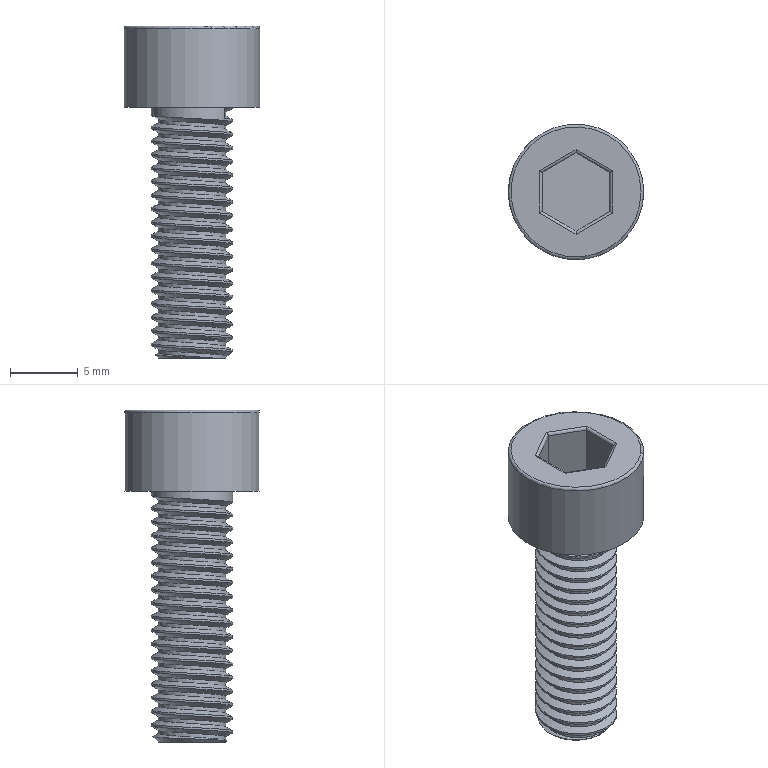Part | STEP file | Tube feed_id174_x_t | 1 solid | 26 faces | box 10 x 10 x 24.5 mm | volume 815.499 mm3 | plane 12 | cylinder 9 | spline 3 | cone 1 | torus 1 | commonest cylinder face diameters 0.4 x6 5 x1 6 x1 10 x1